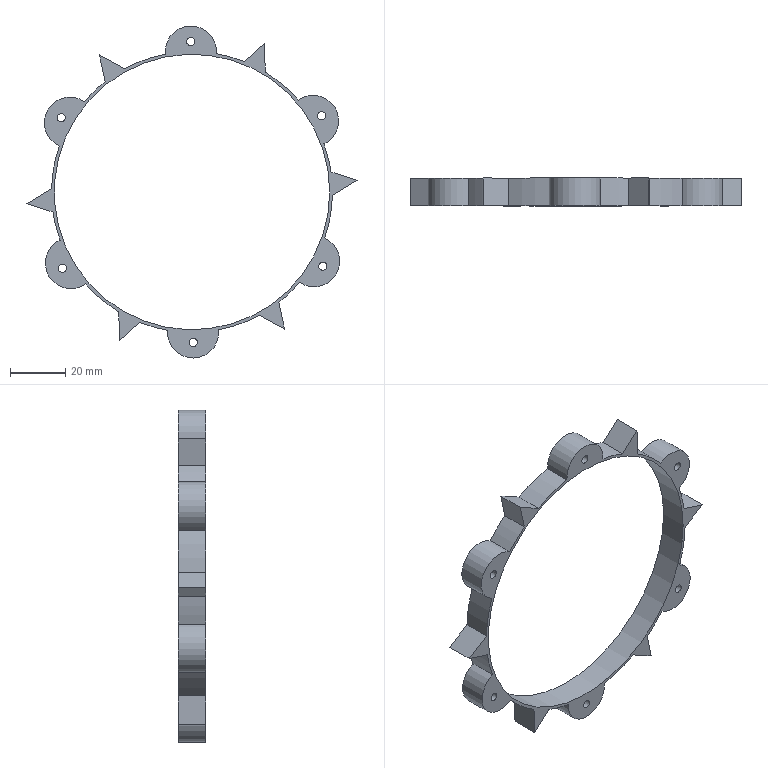Part | NX | features DATUM_CSYS 3, EXTRUDE 2, SKETCH 2 | 1 solid | 39 faces | box 119.85 x 10 x 120.564 mm | volume 13504 mm3 | cylinder 25 | plane 14 | commonest cylinder face diameters 102 x12 3 x6 18.567 x6 100 x1
STEP:
#1=CARTESIAN_POINT('',(-50.984,0.,1.273));
#2=VERTEX_POINT('',#1);
#3=CARTESIAN_POINT('',(-59.925,0.,-4.222));
#4=VERTEX_POINT('',#3);
#5=CARTESIAN_POINT('',(-50.984,0.,1.273));
#6=DIRECTION('',(-0.852,0.,-0.5236));
#7=VECTOR('',#6,1000.);
#8=LINE('',#5,#7);
#9=EDGE_CURVE('',#2,#4,#8,.T.);
#10=ORIENTED_EDGE('',*,*,#9,.T.);
#11=CARTESIAN_POINT('',(-59.925,-10.,-4.222));
#12=VERTEX_POINT('',#11);
#13=CARTESIAN_POINT('',(-59.925,-10.,-4.222));
#14=DIRECTION('',(0.,1.,0.));
#15=VECTOR('',#14,1000.);
#16=LINE('',#13,#15);
#17=EDGE_CURVE('',#12,#4,#16,.T.);
#18=ORIENTED_EDGE('',*,*,#17,.F.);
#19=CARTESIAN_POINT('',(-50.984,-10.,1.273));
#20=VERTEX_POINT('',#19);
#21=CARTESIAN_POINT('',(-50.984,-10.,1.273));
#22=DIRECTION('',(-0.852,0.,-0.5236));
#23=VECTOR('',#22,1000.);
#24=LINE('',#21,#23);
#25=EDGE_CURVE('',#20,#12,#24,.T.);
#26=ORIENTED_EDGE('',*,*,#25,.F.);
#27=CARTESIAN_POINT('',(-50.984,-10.,1.273));
#28=DIRECTION('',(0.,1.,0.));
#29=VECTOR('',#28,1000.);
#30=LINE('',#27,#29);
#31=EDGE_CURVE('',#20,#2,#30,.T.);
#32=ORIENTED_EDGE('',*,*,#31,.T.);
#33=EDGE_LOOP('',(#10,#18,#26,#32));
#34=FACE_BOUND('',#33,.T.);
#35=CARTESIAN_POINT('',(-50.984,-10.,1.273));
#36=DIRECTION('',(0.5236,0.,-0.852));
#37=DIRECTION('',(-0.852,0.,-0.5236));
#38=AXIS2_PLACEMENT_3D('',#35,#36,#37);
#39=PLANE('',#38);
#40=ADVANCED_FACE('',(#34),#39,.F.);
#41=CARTESIAN_POINT('',(-50.476,0.,-7.292));
#42=VERTEX_POINT('',#41);
#43=CARTESIAN_POINT('',(-59.925,0.,-4.222));
#44=DIRECTION('',(0.9511,0.,-0.309));
#45=VECTOR('',#44,1000.);
#46=LINE('',#43,#45);
#47=EDGE_CURVE('',#4,#42,#46,.T.);
#48=ORIENTED_EDGE('',*,*,#47,.T.);
#49=CARTESIAN_POINT('',(-50.476,-10.,-7.292));
#50=VERTEX_POINT('',#49);
#51=CARTESIAN_POINT('',(-50.476,-10.,-7.292));
#52=DIRECTION('',(0.,1.,0.));
#53=VECTOR('',#52,1000.);
#54=LINE('',#51,#53);
#55=EDGE_CURVE('',#50,#42,#54,.T.);
#56=ORIENTED_EDGE('',*,*,#55,.F.);
#57=CARTESIAN_POINT('',(-59.925,-10.,-4.222));
#58=DIRECTION('',(0.9511,0.,-0.309));
#59=VECTOR('',#58,1000.);
#60=LINE('',#57,#59);
#61=EDGE_CURVE('',#12,#50,#60,.T.);
#62=ORIENTED_EDGE('',*,*,#61,.F.);
#63=ORIENTED_EDGE('',*,*,#17,.T.);
#64=EDGE_LOOP('',(#48,#56,#62,#63));
#65=FACE_BOUND('',#64,.T.);
#66=CARTESIAN_POINT('',(-59.925,-10.,-4.222));
#67=DIRECTION('',(0.309,0.,0.9511));
#68=DIRECTION('',(0.9511,0.,-0.309));
#69=AXIS2_PLACEMENT_3D('',#66,#67,#68);
#70=PLANE('',#69);
#71=ADVANCED_FACE('',(#65),#70,.F.);
#72=CARTESIAN_POINT('',(-47.922,0.,-17.449));
#73=VERTEX_POINT('',#72);
#74=CARTESIAN_POINT('',(0.,0.,0.));
#75=DIRECTION('',(0.,-1.,0.));
#76=DIRECTION('',(1.,0.,0.));
#77=AXIS2_PLACEMENT_3D('',#74,#75,#76);
#78=CIRCLE('',#77,51.);
#79=EDGE_CURVE('',#42,#73,#78,.T.);
#80=ORIENTED_EDGE('',*,*,#79,.T.);
#81=CARTESIAN_POINT('',(-47.922,-10.,-17.449));
#82=VERTEX_POINT('',#81);
#83=CARTESIAN_POINT('',(-47.922,-10.,-17.449));
#84=DIRECTION('',(0.,1.,0.));
#85=VECTOR('',#84,1000.);
#86=LINE('',#83,#85);
#87=EDGE_CURVE('',#82,#73,#86,.T.);
#88=ORIENTED_EDGE('',*,*,#87,.F.);
#89=CARTESIAN_POINT('',(0.,-10.,0.));
#90=DIRECTION('',(0.,-1.,0.));
#91=DIRECTION('',(1.,0.,0.));
#92=AXIS2_PLACEMENT_3D('',#89,#90,#91);
#93=CIRCLE('',#92,51.);
#94=EDGE_CURVE('',#50,#82,#93,.T.);
#95=ORIENTED_EDGE('',*,*,#94,.F.);
#96=ORIENTED_EDGE('',*,*,#55,.T.);
#97=EDGE_LOOP('',(#80,#88,#95,#96));
#98=FACE_BOUND('',#97,.T.);
#99=CARTESIAN_POINT('',(0.,-10.,0.));
#100=DIRECTION('',(0.,1.,0.));
#101=DIRECTION('',(0.,0.,1.));
#102=AXIS2_PLACEMENT_3D('',#99,#100,#101);
#103=CYLINDRICAL_SURFACE('',#102,51.);
#104=ADVANCED_FACE('',(#98),#103,.T.);
#105=CARTESIAN_POINT('',(-38.551,0.,-33.388));
#106=VERTEX_POINT('',#105);
#107=CARTESIAN_POINT('',(-43.965,0.,-25.847));
#108=DIRECTION('',(0.,-1.,0.));
#109=DIRECTION('',(-0.5,0.,0.866));
#110=AXIS2_PLACEMENT_3D('',#107,#108,#109);
#111=CIRCLE('',#110,9.283);
#112=EDGE_CURVE('',#73,#106,#111,.T.);
#113=ORIENTED_EDGE('',*,*,#112,.T.);
#114=CARTESIAN_POINT('',(-38.551,-10.,-33.388));
#115=VERTEX_POINT('',#114);
#116=CARTESIAN_POINT('',(-38.551,-10.,-33.388));
#117=DIRECTION('',(0.,1.,0.));
#118=VECTOR('',#117,1000.);
#119=LINE('',#116,#118);
#120=EDGE_CURVE('',#115,#106,#119,.T.);
#121=ORIENTED_EDGE('',*,*,#120,.F.);
#122=CARTESIAN_POINT('',(-43.965,-10.,-25.847));
#123=DIRECTION('',(0.,-1.,0.));
#124=DIRECTION('',(-0.5,0.,0.866));
#125=AXIS2_PLACEMENT_3D('',#122,#123,#124);
#126=CIRCLE('',#125,9.283);
#127=EDGE_CURVE('',#82,#115,#126,.T.);
#128=ORIENTED_EDGE('',*,*,#127,.F.);
#129=ORIENTED_EDGE('',*,*,#87,.T.);
#130=EDGE_LOOP('',(#113,#121,#128,#129));
#131=FACE_BOUND('',#130,.T.);
#132=CARTESIAN_POINT('',(-43.965,-10.,-25.847));
#133=DIRECTION('',(0.,1.,0.));
#134=DIRECTION('',(0.,0.,1.));
#135=AXIS2_PLACEMENT_3D('',#132,#133,#134);
#136=CYLINDRICAL_SURFACE('',#135,9.283);
#137=ADVANCED_FACE('',(#131),#136,.T.);
#138=CARTESIAN_POINT('',(-26.594,0.,-43.517));
#139=VERTEX_POINT('',#138);
#140=CARTESIAN_POINT('',(0.,0.,0.));
#141=DIRECTION('',(0.,-1.,0.));
#142=DIRECTION('',(1.,0.,0.));
#143=AXIS2_PLACEMENT_3D('',#140,#141,#142);
#144=CIRCLE('',#143,51.);
#145=EDGE_CURVE('',#106,#139,#144,.T.);
#146=ORIENTED_EDGE('',*,*,#145,.T.);
#147=CARTESIAN_POINT('',(-26.594,-10.,-43.517));
#148=VERTEX_POINT('',#147);
#149=CARTESIAN_POINT('',(-26.594,-10.,-43.517));
#150=DIRECTION('',(0.,1.,0.));
#151=VECTOR('',#150,1000.);
#152=LINE('',#149,#151);
#153=EDGE_CURVE('',#148,#139,#152,.T.);
#154=ORIENTED_EDGE('',*,*,#153,.F.);
#155=CARTESIAN_POINT('',(0.,-10.,0.));
#156=DIRECTION('',(0.,-1.,0.));
#157=DIRECTION('',(1.,0.,0.));
#158=AXIS2_PLACEMENT_3D('',#155,#156,#157);
#159=CIRCLE('',#158,51.);
#160=EDGE_CURVE('',#115,#148,#159,.T.);
#161=ORIENTED_EDGE('',*,*,#160,.F.);
#162=ORIENTED_EDGE('',*,*,#120,.T.);
#163=EDGE_LOOP('',(#146,#154,#161,#162));
#164=FACE_BOUND('',#163,.T.);
#165=CARTESIAN_POINT('',(0.,-10.,0.));
#166=DIRECTION('',(0.,1.,0.));
#167=DIRECTION('',(0.,0.,1.));
#168=AXIS2_PLACEMENT_3D('',#165,#166,#167);
#169=CYLINDRICAL_SURFACE('',#168,51.);
#170=ADVANCED_FACE('',(#164),#169,.T.);
#171=CARTESIAN_POINT('',(-26.306,0.,-54.007));
#172=VERTEX_POINT('',#171);
#173=CARTESIAN_POINT('',(-26.594,0.,-43.517));
#174=DIRECTION('',(0.02744,0.,-0.9996));
#175=VECTOR('',#174,1000.);
#176=LINE('',#173,#175);
#177=EDGE_CURVE('',#139,#172,#176,.T.);
#178=ORIENTED_EDGE('',*,*,#177,.T.);
#179=CARTESIAN_POINT('',(-26.306,-10.,-54.007));
#180=VERTEX_POINT('',#179);
#181=CARTESIAN_POINT('',(-26.306,-10.,-54.007));
#182=DIRECTION('',(0.,1.,0.));
#183=VECTOR('',#182,1000.);
#184=LINE('',#181,#183);
#185=EDGE_CURVE('',#180,#172,#184,.T.);
#186=ORIENTED_EDGE('',*,*,#185,.F.);
#187=CARTESIAN_POINT('',(-26.594,-10.,-43.517));
#188=DIRECTION('',(0.02744,0.,-0.9996));
#189=VECTOR('',#188,1000.);
#190=LINE('',#187,#189);
#191=EDGE_CURVE('',#148,#180,#190,.T.);
#192=ORIENTED_EDGE('',*,*,#191,.F.);
#193=ORIENTED_EDGE('',*,*,#153,.T.);
#194=EDGE_LOOP('',(#178,#186,#192,#193));
#195=FACE_BOUND('',#194,.T.);
#196=CARTESIAN_POINT('',(-26.594,-10.,-43.517));
#197=DIRECTION('',(0.9996,0.,0.02744));
#198=DIRECTION('',(0.02744,0.,-0.9996));
#199=AXIS2_PLACEMENT_3D('',#196,#197,#198);
#200=PLANE('',#199);
#201=ADVANCED_FACE('',(#195),#200,.F.);
#202=CARTESIAN_POINT('',(-18.923,0.,-47.359));
#203=VERTEX_POINT('',#202);
#204=CARTESIAN_POINT('',(-26.306,0.,-54.007));
#205=DIRECTION('',(0.7431,0.,0.6691));
#206=VECTOR('',#205,1000.);
#207=LINE('',#204,#206);
#208=EDGE_CURVE('',#172,#203,#207,.T.);
#209=ORIENTED_EDGE('',*,*,#208,.T.);
#210=CARTESIAN_POINT('',(-18.923,-10.,-47.359));
#211=VERTEX_POINT('',#210);
#212=CARTESIAN_POINT('',(-18.923,-10.,-47.359));
#213=DIRECTION('',(0.,1.,0.));
#214=VECTOR('',#213,1000.);
#215=LINE('',#212,#214);
#216=EDGE_CURVE('',#211,#203,#215,.T.);
#217=ORIENTED_EDGE('',*,*,#216,.F.);
#218=CARTESIAN_POINT('',(-26.306,-10.,-54.007));
#219=DIRECTION('',(0.7431,0.,0.6691));
#220=VECTOR('',#219,1000.);
#221=LINE('',#218,#220);
#222=EDGE_CURVE('',#180,#211,#221,.T.);
#223=ORIENTED_EDGE('',*,*,#222,.F.);
#224=ORIENTED_EDGE('',*,*,#185,.T.);
#225=EDGE_LOOP('',(#209,#217,#223,#224));
#226=FACE_BOUND('',#225,.T.);
#227=CARTESIAN_POINT('',(-26.306,-10.,-54.007));
#228=DIRECTION('',(-0.6691,0.,0.7431));
#229=DIRECTION('',(0.7431,0.,0.6691));
#230=AXIS2_PLACEMENT_3D('',#227,#228,#229);
#231=PLANE('',#230);
#232=ADVANCED_FACE('',(#226),#231,.F.);
#233=CARTESIAN_POINT('',(-8.85,0.,-50.226));
#234=VERTEX_POINT('',#233);
#235=CARTESIAN_POINT('',(0.,0.,0.));
#236=DIRECTION('',(0.,-1.,0.));
#237=DIRECTION('',(1.,0.,0.));
#238=AXIS2_PLACEMENT_3D('',#235,#236,#237);
#239=CIRCLE('',#238,51.);
#240=EDGE_CURVE('',#203,#234,#239,.T.);
#241=ORIENTED_EDGE('',*,*,#240,.T.);
#242=CARTESIAN_POINT('',(-8.85,-10.,-50.226));
#243=VERTEX_POINT('',#242);
#244=CARTESIAN_POINT('',(-8.85,-10.,-50.226));
#245=DIRECTION('',(0.,1.,0.));
#246=VECTOR('',#245,1000.);
#247=LINE('',#244,#246);
#248=EDGE_CURVE('',#243,#234,#247,.T.);
#249=ORIENTED_EDGE('',*,*,#248,.F.);
#250=CARTESIAN_POINT('',(0.,-10.,0.));
#251=DIRECTION('',(0.,-1.,0.));
#252=DIRECTION('',(1.,0.,0.));
#253=AXIS2_PLACEMENT_3D('',#250,#251,#252);
#254=CIRCLE('',#253,51.);
#255=EDGE_CURVE('',#211,#243,#254,.T.);
#256=ORIENTED_EDGE('',*,*,#255,.F.);
#257=ORIENTED_EDGE('',*,*,#216,.T.);
#258=EDGE_LOOP('',(#241,#249,#256,#257));
#259=FACE_BOUND('',#258,.T.);
#260=CARTESIAN_POINT('',(0.,-10.,0.));
#261=DIRECTION('',(0.,1.,0.));
#262=DIRECTION('',(0.,0.,1.));
#263=AXIS2_PLACEMENT_3D('',#260,#261,#262);
#264=CYLINDRICAL_SURFACE('',#263,51.);
#265=ADVANCED_FACE('',(#259),#264,.T.);
#266=CARTESIAN_POINT('',(9.64,0.,-50.081));
#267=VERTEX_POINT('',#266);
#268=CARTESIAN_POINT('',(0.4017,0.,-50.998));
#269=DIRECTION('',(0.,-1.,0.));
#270=DIRECTION('',(-1.,0.,0.));
#271=AXIS2_PLACEMENT_3D('',#268,#269,#270);
#272=CIRCLE('',#271,9.283);
#273=EDGE_CURVE('',#234,#267,#272,.T.);
#274=ORIENTED_EDGE('',*,*,#273,.T.);
#275=CARTESIAN_POINT('',(9.64,-10.,-50.081));
#276=VERTEX_POINT('',#275);
#277=CARTESIAN_POINT('',(9.64,-10.,-50.081));
#278=DIRECTION('',(0.,1.,0.));
#279=VECTOR('',#278,1000.);
#280=LINE('',#277,#279);
#281=EDGE_CURVE('',#276,#267,#280,.T.);
#282=ORIENTED_EDGE('',*,*,#281,.F.);
#283=CARTESIAN_POINT('',(0.4017,-10.,-50.998));
#284=DIRECTION('',(0.,-1.,0.));
#285=DIRECTION('',(-1.,0.,0.));
#286=AXIS2_PLACEMENT_3D('',#283,#284,#285);
#287=CIRCLE('',#286,9.283);
#288=EDGE_CURVE('',#243,#276,#287,.T.);
#289=ORIENTED_EDGE('',*,*,#288,.F.);
#290=ORIENTED_EDGE('',*,*,#248,.T.);
#291=EDGE_LOOP('',(#274,#282,#289,#290));
#292=FACE_BOUND('',#291,.T.);
#293=CARTESIAN_POINT('',(0.4017,-10.,-50.998));
#294=DIRECTION('',(0.,1.,0.));
#295=DIRECTION('',(0.,0.,1.));
#296=AXIS2_PLACEMENT_3D('',#293,#294,#295);
#297=CYLINDRICAL_SURFACE('',#296,9.283);
#298=ADVANCED_FACE('',(#292),#297,.T.);
#299=CARTESIAN_POINT('',(24.39,0.,-44.79));
#300=VERTEX_POINT('',#299);
#301=CARTESIAN_POINT('',(0.,0.,0.));
#302=DIRECTION('',(0.,-1.,0.));
#303=DIRECTION('',(1.,0.,0.));
#304=AXIS2_PLACEMENT_3D('',#301,#302,#303);
#305=CIRCLE('',#304,51.);
#306=EDGE_CURVE('',#267,#300,#305,.T.);
#307=ORIENTED_EDGE('',*,*,#306,.T.);
#308=CARTESIAN_POINT('',(24.39,-10.,-44.79));
#309=VERTEX_POINT('',#308);
#310=CARTESIAN_POINT('',(24.39,-10.,-44.79));
#311=DIRECTION('',(0.,1.,0.));
#312=VECTOR('',#311,1000.);
#313=LINE('',#310,#312);
#314=EDGE_CURVE('',#309,#300,#313,.T.);
#315=ORIENTED_EDGE('',*,*,#314,.F.);
#316=CARTESIAN_POINT('',(0.,-10.,0.));
#317=DIRECTION('',(0.,-1.,0.));
#318=DIRECTION('',(1.,0.,0.));
#319=AXIS2_PLACEMENT_3D('',#316,#317,#318);
#320=CIRCLE('',#319,51.);
#321=EDGE_CURVE('',#276,#309,#320,.T.);
#322=ORIENTED_EDGE('',*,*,#321,.F.);
#323=ORIENTED_EDGE('',*,*,#281,.T.);
#324=EDGE_LOOP('',(#307,#315,#322,#323));
#325=FACE_BOUND('',#324,.T.);
#326=CARTESIAN_POINT('',(0.,-10.,0.));
#327=DIRECTION('',(0.,1.,0.));
#328=DIRECTION('',(0.,0.,1.));
#329=AXIS2_PLACEMENT_3D('',#326,#327,#328);
#330=CYLINDRICAL_SURFACE('',#329,51.);
#331=ADVANCED_FACE('',(#325),#330,.T.);
#332=CARTESIAN_POINT('',(33.619,0.,-49.786));
#333=VERTEX_POINT('',#332);
#334=CARTESIAN_POINT('',(24.39,0.,-44.79));
#335=DIRECTION('',(0.8794,0.,-0.476));
#336=VECTOR('',#335,1000.);
#337=LINE('',#334,#336);
#338=EDGE_CURVE('',#300,#333,#337,.T.);
#339=ORIENTED_EDGE('',*,*,#338,.T.);
#340=CARTESIAN_POINT('',(33.619,-10.,-49.786));
#341=VERTEX_POINT('',#340);
#342=CARTESIAN_POINT('',(33.619,-10.,-49.786));
#343=DIRECTION('',(0.,1.,0.));
#344=VECTOR('',#343,1000.);
#345=LINE('',#342,#344);
#346=EDGE_CURVE('',#341,#333,#345,.T.);
#347=ORIENTED_EDGE('',*,*,#346,.F.);
#348=CARTESIAN_POINT('',(24.39,-10.,-44.79));
#349=DIRECTION('',(0.8794,0.,-0.476));
#350=VECTOR('',#349,1000.);
#351=LINE('',#348,#350);
#352=EDGE_CURVE('',#309,#341,#351,.T.);
#353=ORIENTED_EDGE('',*,*,#352,.F.);
#354=ORIENTED_EDGE('',*,*,#314,.T.);
#355=EDGE_LOOP('',(#339,#347,#353,#354));
#356=FACE_BOUND('',#355,.T.);
#357=CARTESIAN_POINT('',(24.39,-10.,-44.79));
#358=DIRECTION('',(0.476,0.,0.8794));
#359=DIRECTION('',(0.8794,0.,-0.476));
#360=AXIS2_PLACEMENT_3D('',#357,#358,#359);
#361=PLANE('',#360);
#362=ADVANCED_FACE('',(#356),#361,.F.);
#363=CARTESIAN_POINT('',(31.553,0.,-40.068));
#364=VERTEX_POINT('',#363);
#365=CARTESIAN_POINT('',(33.619,0.,-49.786));
#366=DIRECTION('',(-0.2079,0.,0.9781));
#367=VECTOR('',#366,1000.);
#368=LINE('',#365,#367);
#369=EDGE_CURVE('',#333,#364,#368,.T.);
#370=ORIENTED_EDGE('',*,*,#369,.T.);
#371=CARTESIAN_POINT('',(31.553,-10.,-40.068));
#372=VERTEX_POINT('',#371);
#373=CARTESIAN_POINT('',(31.553,-10.,-40.068));
#374=DIRECTION('',(0.,1.,0.));
#375=VECTOR('',#374,1000.);
#376=LINE('',#373,#375);
#377=EDGE_CURVE('',#372,#364,#376,.T.);
#378=ORIENTED_EDGE('',*,*,#377,.F.);
#379=CARTESIAN_POINT('',(33.619,-10.,-49.786));
#380=DIRECTION('',(-0.2079,0.,0.9781));
#381=VECTOR('',#380,1000.);
#382=LINE('',#379,#381);
#383=EDGE_CURVE('',#341,#372,#382,.T.);
#384=ORIENTED_EDGE('',*,*,#383,.F.);
#385=ORIENTED_EDGE('',*,*,#346,.T.);
#386=EDGE_LOOP('',(#370,#378,#384,#385));
#387=FACE_BOUND('',#386,.T.);
#388=CARTESIAN_POINT('',(33.619,-10.,-49.786));
#389=DIRECTION('',(-0.9781,0.,-0.2079));
#390=DIRECTION('',(-0.2079,0.,0.9781));
#391=AXIS2_PLACEMENT_3D('',#388,#389,#390);
#392=PLANE('',#391);
#393=ADVANCED_FACE('',(#387),#392,.F.);
#394=CARTESIAN_POINT('',(39.073,0.,-32.777));
#395=VERTEX_POINT('',#394);
#396=CARTESIAN_POINT('',(0.,0.,0.));
#397=DIRECTION('',(0.,-1.,0.));
#398=DIRECTION('',(1.,0.,0.));
#399=AXIS2_PLACEMENT_3D('',#396,#397,#398);
#400=CIRCLE('',#399,51.);
#401=EDGE_CURVE('',#364,#395,#400,.T.);
#402=ORIENTED_EDGE('',*,*,#401,.T.);
#403=CARTESIAN_POINT('',(39.073,-10.,-32.777));
#404=VERTEX_POINT('',#403);
#405=CARTESIAN_POINT('',(39.073,-10.,-32.777));
#406=DIRECTION('',(0.,1.,0.));
#407=VECTOR('',#406,1000.);
#408=LINE('',#405,#407);
#409=EDGE_CURVE('',#404,#395,#408,.T.);
#410=ORIENTED_EDGE('',*,*,#409,.F.);
#411=CARTESIAN_POINT('',(0.,-10.,0.));
#412=DIRECTION('',(0.,-1.,0.));
#413=DIRECTION('',(1.,0.,0.));
#414=AXIS2_PLACEMENT_3D('',#411,#412,#413);
#415=CIRCLE('',#414,51.);
#416=EDGE_CURVE('',#372,#404,#415,.T.);
#417=ORIENTED_EDGE('',*,*,#416,.F.);
#418=ORIENTED_EDGE('',*,*,#377,.T.);
#419=EDGE_LOOP('',(#402,#410,#417,#418));
#420=FACE_BOUND('',#419,.T.);
#421=CARTESIAN_POINT('',(0.,-10.,0.));
#422=DIRECTION('',(0.,1.,0.));
#423=DIRECTION('',(0.,0.,1.));
#424=AXIS2_PLACEMENT_3D('',#421,#422,#423);
#425=CYLINDRICAL_SURFACE('',#424,51.);
#426=ADVANCED_FACE('',(#420),#425,.T.);
#427=CARTESIAN_POINT('',(48.191,0.,-16.692));
#428=VERTEX_POINT('',#427);
#429=CARTESIAN_POINT('',(44.367,0.,-25.151));
#430=DIRECTION('',(0.,-1.,0.));
#431=DIRECTION('',(-0.5,0.,-0.866));
#432=AXIS2_PLACEMENT_3D('',#429,#430,#431);
#433=CIRCLE('',#432,9.283);
#434=EDGE_CURVE('',#395,#428,#433,.T.);
#435=ORIENTED_EDGE('',*,*,#434,.T.);
#436=CARTESIAN_POINT('',(48.191,-10.,-16.692));
#437=VERTEX_POINT('',#436);
#438=CARTESIAN_POINT('',(48.191,-10.,-16.692));
#439=DIRECTION('',(0.,1.,0.));
#440=VECTOR('',#439,1000.);
#441=LINE('',#438,#440);
#442=EDGE_CURVE('',#437,#428,#441,.T.);
#443=ORIENTED_EDGE('',*,*,#442,.F.);
#444=CARTESIAN_POINT('',(44.367,-10.,-25.151));
#445=DIRECTION('',(0.,-1.,0.));
#446=DIRECTION('',(-0.5,0.,-0.866));
#447=AXIS2_PLACEMENT_3D('',#444,#445,#446);
#448=CIRCLE('',#447,9.283);
#449=EDGE_CURVE('',#404,#437,#448,.T.);
#450=ORIENTED_EDGE('',*,*,#449,.F.);
#451=ORIENTED_EDGE('',*,*,#409,.T.);
#452=EDGE_LOOP('',(#435,#443,#450,#451));
#453=FACE_BOUND('',#452,.T.);
#454=CARTESIAN_POINT('',(44.367,-10.,-25.151));
#455=DIRECTION('',(0.,1.,0.));
#456=DIRECTION('',(0.,0.,1.));
#457=AXIS2_PLACEMENT_3D('',#454,#455,#456);
#458=CYLINDRICAL_SURFACE('',#457,9.283);
#459=ADVANCED_FACE('',(#453),#458,.T.);
#460=CARTESIAN_POINT('',(50.984,0.,-1.273));
#461=VERTEX_POINT('',#460);
#462=CARTESIAN_POINT('',(0.,0.,0.));
#463=DIRECTION('',(0.,-1.,0.));
#464=DIRECTION('',(1.,0.,0.));
#465=AXIS2_PLACEMENT_3D('',#462,#463,#464);
#466=CIRCLE('',#465,51.);
#467=EDGE_CURVE('',#428,#461,#466,.T.);
#468=ORIENTED_EDGE('',*,*,#467,.T.);
#469=CARTESIAN_POINT('',(50.984,-10.,-1.273));
#470=VERTEX_POINT('',#469);
#471=CARTESIAN_POINT('',(50.984,-10.,-1.273));
#472=DIRECTION('',(0.,1.,0.));
#473=VECTOR('',#472,1000.);
#474=LINE('',#471,#473);
#475=EDGE_CURVE('',#470,#461,#474,.T.);
#476=ORIENTED_EDGE('',*,*,#475,.F.);
#477=CARTESIAN_POINT('',(0.,-10.,0.));
#478=DIRECTION('',(0.,-1.,0.));
#479=DIRECTION('',(1.,0.,0.));
#480=AXIS2_PLACEMENT_3D('',#477,#478,#479);
#481=CIRCLE('',#480,51.);
#482=EDGE_CURVE('',#437,#470,#481,.T.);
#483=ORIENTED_EDGE('',*,*,#482,.F.);
#484=ORIENTED_EDGE('',*,*,#442,.T.);
#485=EDGE_LOOP('',(#468,#476,#483,#484));
#486=FACE_BOUND('',#485,.T.);
#487=CARTESIAN_POINT('',(0.,-10.,0.));
#488=DIRECTION('',(0.,1.,0.));
#489=DIRECTION('',(0.,0.,1.));
#490=AXIS2_PLACEMENT_3D('',#487,#488,#489);
#491=CYLINDRICAL_SURFACE('',#490,51.);
#492=ADVANCED_FACE('',(#486),#491,.T.);
#493=CARTESIAN_POINT('',(59.925,0.,4.222));
#494=VERTEX_POINT('',#493);
#495=CARTESIAN_POINT('',(50.984,0.,-1.273));
#496=DIRECTION('',(0.852,0.,0.5236));
#497=VECTOR('',#496,1000.);
#498=LINE('',#495,#497);
#499=EDGE_CURVE('',#461,#494,#498,.T.);
#500=ORIENTED_EDGE('',*,*,#499,.T.);
#501=CARTESIAN_POINT('',(59.925,-10.,4.222));
#502=VERTEX_POINT('',#501);
#503=CARTESIAN_POINT('',(59.925,-10.,4.222));
#504=DIRECTION('',(0.,1.,0.));
#505=VECTOR('',#504,1000.);
#506=LINE('',#503,#505);
#507=EDGE_CURVE('',#502,#494,#506,.T.);
#508=ORIENTED_EDGE('',*,*,#507,.F.);
#509=CARTESIAN_POINT('',(50.984,-10.,-1.273));
#510=DIRECTION('',(0.852,0.,0.5236));
#511=VECTOR('',#510,1000.);
#512=LINE('',#509,#511);
#513=EDGE_CURVE('',#470,#502,#512,.T.);
#514=ORIENTED_EDGE('',*,*,#513,.F.);
#515=ORIENTED_EDGE('',*,*,#475,.T.);
#516=EDGE_LOOP('',(#500,#508,#514,#515));
#517=FACE_BOUND('',#516,.T.);
#518=CARTESIAN_POINT('',(50.984,-10.,-1.273));
#519=DIRECTION('',(-0.5236,0.,0.852));
#520=DIRECTION('',(0.852,0.,0.5236));
#521=AXIS2_PLACEMENT_3D('',#518,#519,#520);
#522=PLANE('',#521);
#523=ADVANCED_FACE('',(#517),#522,.F.);
#524=CARTESIAN_POINT('',(50.476,0.,7.292));
#525=VERTEX_POINT('',#524);
#526=CARTESIAN_POINT('',(59.925,0.,4.222));
#527=DIRECTION('',(-0.9511,0.,0.309));
#528=VECTOR('',#527,1000.);
#529=LINE('',#526,#528);
#530=EDGE_CURVE('',#494,#525,#529,.T.);
#531=ORIENTED_EDGE('',*,*,#530,.T.);
#532=CARTESIAN_POINT('',(50.476,-10.,7.292));
#533=VERTEX_POINT('',#532);
#534=CARTESIAN_POINT('',(50.476,-10.,7.292));
#535=DIRECTION('',(0.,1.,0.));
#536=VECTOR('',#535,1000.);
#537=LINE('',#534,#536);
#538=EDGE_CURVE('',#533,#525,#537,.T.);
#539=ORIENTED_EDGE('',*,*,#538,.F.);
#540=CARTESIAN_POINT('',(59.925,-10.,4.222));
#541=DIRECTION('',(-0.9511,0.,0.309));
#542=VECTOR('',#541,1000.);
#543=LINE('',#540,#542);
#544=EDGE_CURVE('',#502,#533,#543,.T.);
#545=ORIENTED_EDGE('',*,*,#544,.F.);
#546=ORIENTED_EDGE('',*,*,#507,.T.);
#547=EDGE_LOOP('',(#531,#539,#545,#546));
#548=FACE_BOUND('',#547,.T.);
#549=CARTESIAN_POINT('',(59.925,-10.,4.222));
#550=DIRECTION('',(-0.309,0.,-0.9511));
#551=DIRECTION('',(-0.9511,0.,0.309));
#552=AXIS2_PLACEMENT_3D('',#549,#550,#551);
#553=PLANE('',#552);
#554=ADVANCED_FACE('',(#548),#553,.F.);
#555=CARTESIAN_POINT('',(47.922,0.,17.449));
#556=VERTEX_POINT('',#555);
#557=CARTESIAN_POINT('',(0.,0.,0.));
#558=DIRECTION('',(0.,-1.,0.));
#559=DIRECTION('',(1.,0.,0.));
#560=AXIS2_PLACEMENT_3D('',#557,#558,#559);
#561=CIRCLE('',#560,51.);
#562=EDGE_CURVE('',#525,#556,#561,.T.);
#563=ORIENTED_EDGE('',*,*,#562,.T.);
#564=CARTESIAN_POINT('',(47.922,-10.,17.449));
#565=VERTEX_POINT('',#564);
#566=CARTESIAN_POINT('',(47.922,-10.,17.449));
#567=DIRECTION('',(0.,1.,0.));
#568=VECTOR('',#567,1000.);
#569=LINE('',#566,#568);
#570=EDGE_CURVE('',#565,#556,#569,.T.);
#571=ORIENTED_EDGE('',*,*,#570,.F.);
#572=CARTESIAN_POINT('',(0.,-10.,0.));
#573=DIRECTION('',(0.,-1.,0.));
#574=DIRECTION('',(1.,0.,0.));
#575=AXIS2_PLACEMENT_3D('',#572,#573,#574);
#576=CIRCLE('',#575,51.);
#577=EDGE_CURVE('',#533,#565,#576,.T.);
#578=ORIENTED_EDGE('',*,*,#577,.F.);
#579=ORIENTED_EDGE('',*,*,#538,.T.);
#580=EDGE_LOOP('',(#563,#571,#578,#579));
#581=FACE_BOUND('',#580,.T.);
#582=CARTESIAN_POINT('',(0.,-10.,0.));
#583=DIRECTION('',(0.,1.,0.));
#584=DIRECTION('',(0.,0.,1.));
#585=AXIS2_PLACEMENT_3D('',#582,#583,#584);
#586=CYLINDRICAL_SURFACE('',#585,51.);
#587=ADVANCED_FACE('',(#581),#586,.T.);
#588=CARTESIAN_POINT('',(38.551,0.,33.388));
#589=VERTEX_POINT('',#588);
#590=CARTESIAN_POINT('',(43.965,0.,25.847));
#591=DIRECTION('',(0.,-1.,0.));
#592=DIRECTION('',(0.5,0.,-0.866));
#593=AXIS2_PLACEMENT_3D('',#590,#591,#592);
#594=CIRCLE('',#593,9.283);
#595=EDGE_CURVE('',#556,#589,#594,.T.);
#596=ORIENTED_EDGE('',*,*,#595,.T.);
#597=CARTESIAN_POINT('',(38.551,-10.,33.388));
#598=VERTEX_POINT('',#597);
#599=CARTESIAN_POINT('',(38.551,-10.,33.388));
#600=DIRECTION('',(0.,1.,0.));
#601=VECTOR('',#600,1000.);
#602=LINE('',#599,#601);
#603=EDGE_CURVE('',#598,#589,#602,.T.);
#604=ORIENTED_EDGE('',*,*,#603,.F.);
#605=CARTESIAN_POINT('',(43.965,-10.,25.847));
#606=DIRECTION('',(0.,-1.,0.));
#607=DIRECTION('',(0.5,0.,-0.866));
#608=AXIS2_PLACEMENT_3D('',#605,#606,#607);
#609=CIRCLE('',#608,9.283);
#610=EDGE_CURVE('',#565,#598,#609,.T.);
#611=ORIENTED_EDGE('',*,*,#610,.F.);
#612=ORIENTED_EDGE('',*,*,#570,.T.);
#613=EDGE_LOOP('',(#596,#604,#611,#612));
#614=FACE_BOUND('',#613,.T.);
#615=CARTESIAN_POINT('',(43.965,-10.,25.847));
#616=DIRECTION('',(0.,1.,0.));
#617=DIRECTION('',(0.,0.,1.));
#618=AXIS2_PLACEMENT_3D('',#615,#616,#617);
#619=CYLINDRICAL_SURFACE('',#618,9.283);
#620=ADVANCED_FACE('',(#614),#619,.T.);
#621=CARTESIAN_POINT('',(26.594,0.,43.517));
#622=VERTEX_POINT('',#621);
#623=CARTESIAN_POINT('',(0.,0.,0.));
#624=DIRECTION('',(0.,-1.,0.));
#625=DIRECTION('',(1.,0.,0.));
#626=AXIS2_PLACEMENT_3D('',#623,#624,#625);
#627=CIRCLE('',#626,51.);
#628=EDGE_CURVE('',#589,#622,#627,.T.);
#629=ORIENTED_EDGE('',*,*,#628,.T.);
#630=CARTESIAN_POINT('',(26.594,-10.,43.517));
#631=VERTEX_POINT('',#630);
#632=CARTESIAN_POINT('',(26.594,-10.,43.517));
#633=DIRECTION('',(0.,1.,0.));
#634=VECTOR('',#633,1000.);
#635=LINE('',#632,#634);
#636=EDGE_CURVE('',#631,#622,#635,.T.);
#637=ORIENTED_EDGE('',*,*,#636,.F.);
#638=CARTESIAN_POINT('',(0.,-10.,0.));
#639=DIRECTION('',(0.,-1.,0.));
#640=DIRECTION('',(1.,0.,0.));
#641=AXIS2_PLACEMENT_3D('',#638,#639,#640);
#642=CIRCLE('',#641,51.);
#643=EDGE_CURVE('',#598,#631,#642,.T.);
#644=ORIENTED_EDGE('',*,*,#643,.F.);
#645=ORIENTED_EDGE('',*,*,#603,.T.);
#646=EDGE_LOOP('',(#629,#637,#644,#645));
#647=FACE_BOUND('',#646,.T.);
#648=CARTESIAN_POINT('',(0.,-10.,0.));
#649=DIRECTION('',(0.,1.,0.));
#650=DIRECTION('',(0.,0.,1.));
#651=AXIS2_PLACEMENT_3D('',#648,#649,#650);
#652=CYLINDRICAL_SURFACE('',#651,51.);
#653=ADVANCED_FACE('',(#647),#652,.T.);
#654=CARTESIAN_POINT('',(26.306,0.,54.007));
#655=VERTEX_POINT('',#654);
#656=CARTESIAN_POINT('',(26.594,0.,43.517));
#657=DIRECTION('',(-0.02744,0.,0.9996));
#658=VECTOR('',#657,1000.);
#659=LINE('',#656,#658);
#660=EDGE_CURVE('',#622,#655,#659,.T.);
#661=ORIENTED_EDGE('',*,*,#660,.T.);
#662=CARTESIAN_POINT('',(26.306,-10.,54.007));
#663=VERTEX_POINT('',#662);
#664=CARTESIAN_POINT('',(26.306,-10.,54.007));
#665=DIRECTION('',(0.,1.,0.));
#666=VECTOR('',#665,1000.);
#667=LINE('',#664,#666);
#668=EDGE_CURVE('',#663,#655,#667,.T.);
#669=ORIENTED_EDGE('',*,*,#668,.F.);
#670=CARTESIAN_POINT('',(26.594,-10.,43.517));
#671=DIRECTION('',(-0.02744,0.,0.9996));
#672=VECTOR('',#671,1000.);
#673=LINE('',#670,#672);
#674=EDGE_CURVE('',#631,#663,#673,.T.);
#675=ORIENTED_EDGE('',*,*,#674,.F.);
#676=ORIENTED_EDGE('',*,*,#636,.T.);
#677=EDGE_LOOP('',(#661,#669,#675,#676));
#678=FACE_BOUND('',#677,.T.);
#679=CARTESIAN_POINT('',(26.594,-10.,43.517));
#680=DIRECTION('',(-0.9996,0.,-0.02744));
#681=DIRECTION('',(-0.02744,0.,0.9996));
#682=AXIS2_PLACEMENT_3D('',#679,#680,#681);
#683=PLANE('',#682);
#684=ADVANCED_FACE('',(#678),#683,.F.);
#685=CARTESIAN_POINT('',(18.923,0.,47.359));
#686=VERTEX_POINT('',#685);
#687=CARTESIAN_POINT('',(26.306,0.,54.007));
#688=DIRECTION('',(-0.7431,0.,-0.6691));
#689=VECTOR('',#688,1000.);
#690=LINE('',#687,#689);
#691=EDGE_CURVE('',#655,#686,#690,.T.);
#692=ORIENTED_EDGE('',*,*,#691,.T.);
#693=CARTESIAN_POINT('',(18.923,-10.,47.359));
#694=VERTEX_POINT('',#693);
#695=CARTESIAN_POINT('',(18.923,-10.,47.359));
#696=DIRECTION('',(0.,1.,0.));
#697=VECTOR('',#696,1000.);
#698=LINE('',#695,#697);
#699=EDGE_CURVE('',#694,#686,#698,.T.);
#700=ORIENTED_EDGE('',*,*,#699,.F.);
#701=CARTESIAN_POINT('',(26.306,-10.,54.007));
#702=DIRECTION('',(-0.7431,0.,-0.6691));
#703=VECTOR('',#702,1000.);
#704=LINE('',#701,#703);
#705=EDGE_CURVE('',#663,#694,#704,.T.);
#706=ORIENTED_EDGE('',*,*,#705,.F.);
#707=ORIENTED_EDGE('',*,*,#668,.T.);
#708=EDGE_LOOP('',(#692,#700,#706,#707));
#709=FACE_BOUND('',#708,.T.);
#710=CARTESIAN_POINT('',(26.306,-10.,54.007));
#711=DIRECTION('',(0.6691,0.,-0.7431));
#712=DIRECTION('',(-0.7431,0.,-0.6691));
#713=AXIS2_PLACEMENT_3D('',#710,#711,#712);
#714=PLANE('',#713);
#715=ADVANCED_FACE('',(#709),#714,.F.);
#716=CARTESIAN_POINT('',(8.85,0.,50.226));
#717=VERTEX_POINT('',#716);
#718=CARTESIAN_POINT('',(0.,0.,0.));
#719=DIRECTION('',(0.,-1.,0.));
#720=DIRECTION('',(1.,0.,0.));
#721=AXIS2_PLACEMENT_3D('',#718,#719,#720);
#722=CIRCLE('',#721,51.);
#723=EDGE_CURVE('',#686,#717,#722,.T.);
#724=ORIENTED_EDGE('',*,*,#723,.T.);
#725=CARTESIAN_POINT('',(8.85,-10.,50.226));
#726=VERTEX_POINT('',#725);
#727=CARTESIAN_POINT('',(8.85,-10.,50.226));
#728=DIRECTION('',(0.,1.,0.));
#729=VECTOR('',#728,1000.);
#730=LINE('',#727,#729);
#731=EDGE_CURVE('',#726,#717,#730,.T.);
#732=ORIENTED_EDGE('',*,*,#731,.F.);
#733=CARTESIAN_POINT('',(0.,-10.,0.));
#734=DIRECTION('',(0.,-1.,0.));
#735=DIRECTION('',(1.,0.,0.));
#736=AXIS2_PLACEMENT_3D('',#733,#734,#735);
#737=CIRCLE('',#736,51.);
#738=EDGE_CURVE('',#694,#726,#737,.T.);
#739=ORIENTED_EDGE('',*,*,#738,.F.);
#740=ORIENTED_EDGE('',*,*,#699,.T.);
#741=EDGE_LOOP('',(#724,#732,#739,#740));
#742=FACE_BOUND('',#741,.T.);
#743=CARTESIAN_POINT('',(0.,-10.,0.));
#744=DIRECTION('',(0.,1.,0.));
#745=DIRECTION('',(0.,0.,1.));
#746=AXIS2_PLACEMENT_3D('',#743,#744,#745);
#747=CYLINDRICAL_SURFACE('',#746,51.);
#748=ADVANCED_FACE('',(#742),#747,.T.);
#749=CARTESIAN_POINT('',(-9.64,0.,50.081));
#750=VERTEX_POINT('',#749);
#751=CARTESIAN_POINT('',(-0.4017,0.,50.998));
#752=DIRECTION('',(0.,-1.,0.));
#753=DIRECTION('',(1.,0.,0.));
#754=AXIS2_PLACEMENT_3D('',#751,#752,#753);
#755=CIRCLE('',#754,9.283);
#756=EDGE_CURVE('',#717,#750,#755,.T.);
#757=ORIENTED_EDGE('',*,*,#756,.T.);
#758=CARTESIAN_POINT('',(-9.64,-10.,50.081));
#759=VERTEX_POINT('',#758);
#760=CARTESIAN_POINT('',(-9.64,-10.,50.081));
#761=DIRECTION('',(0.,1.,0.));
#762=VECTOR('',#761,1000.);
#763=LINE('',#760,#762);
#764=EDGE_CURVE('',#759,#750,#763,.T.);
#765=ORIENTED_EDGE('',*,*,#764,.F.);
#766=CARTESIAN_POINT('',(-0.4017,-10.,50.998));
#767=DIRECTION('',(0.,-1.,0.));
#768=DIRECTION('',(1.,0.,0.));
#769=AXIS2_PLACEMENT_3D('',#766,#767,#768);
#770=CIRCLE('',#769,9.283);
#771=EDGE_CURVE('',#726,#759,#770,.T.);
#772=ORIENTED_EDGE('',*,*,#771,.F.);
#773=ORIENTED_EDGE('',*,*,#731,.T.);
#774=EDGE_LOOP('',(#757,#765,#772,#773));
#775=FACE_BOUND('',#774,.T.);
#776=CARTESIAN_POINT('',(-0.4017,-10.,50.998));
#777=DIRECTION('',(0.,1.,0.));
#778=DIRECTION('',(0.,0.,1.));
#779=AXIS2_PLACEMENT_3D('',#776,#777,#778);
#780=CYLINDRICAL_SURFACE('',#779,9.283);
#781=ADVANCED_FACE('',(#775),#780,.T.);
#782=CARTESIAN_POINT('',(-24.39,0.,44.79));
#783=VERTEX_POINT('',#782);
#784=CARTESIAN_POINT('',(0.,0.,0.));
#785=DIRECTION('',(0.,-1.,0.));
#786=DIRECTION('',(1.,0.,0.));
#787=AXIS2_PLACEMENT_3D('',#784,#785,#786);
#788=CIRCLE('',#787,51.);
#789=EDGE_CURVE('',#750,#783,#788,.T.);
#790=ORIENTED_EDGE('',*,*,#789,.T.);
#791=CARTESIAN_POINT('',(-24.39,-10.,44.79));
#792=VERTEX_POINT('',#791);
#793=CARTESIAN_POINT('',(-24.39,-10.,44.79));
#794=DIRECTION('',(0.,1.,0.));
#795=VECTOR('',#794,1000.);
#796=LINE('',#793,#795);
#797=EDGE_CURVE('',#792,#783,#796,.T.);
#798=ORIENTED_EDGE('',*,*,#797,.F.);
#799=CARTESIAN_POINT('',(0.,-10.,0.));
#800=DIRECTION('',(0.,-1.,0.));
#801=DIRECTION('',(1.,0.,0.));
#802=AXIS2_PLACEMENT_3D('',#799,#800,#801);
#803=CIRCLE('',#802,51.);
#804=EDGE_CURVE('',#759,#792,#803,.T.);
#805=ORIENTED_EDGE('',*,*,#804,.F.);
#806=ORIENTED_EDGE('',*,*,#764,.T.);
#807=EDGE_LOOP('',(#790,#798,#805,#806));
#808=FACE_BOUND('',#807,.T.);
#809=CARTESIAN_POINT('',(0.,-10.,0.));
#810=DIRECTION('',(0.,1.,0.));
#811=DIRECTION('',(0.,0.,1.));
#812=AXIS2_PLACEMENT_3D('',#809,#810,#811);
#813=CYLINDRICAL_SURFACE('',#812,51.);
#814=ADVANCED_FACE('',(#808),#813,.T.);
#815=CARTESIAN_POINT('',(-33.619,0.,49.786));
#816=VERTEX_POINT('',#815);
#817=CARTESIAN_POINT('',(-24.39,0.,44.79));
#818=DIRECTION('',(-0.8794,0.,0.476));
#819=VECTOR('',#818,1000.);
#820=LINE('',#817,#819);
#821=EDGE_CURVE('',#783,#816,#820,.T.);
#822=ORIENTED_EDGE('',*,*,#821,.T.);
#823=CARTESIAN_POINT('',(-33.619,-10.,49.786));
#824=VERTEX_POINT('',#823);
#825=CARTESIAN_POINT('',(-33.619,-10.,49.786));
#826=DIRECTION('',(0.,1.,0.));
#827=VECTOR('',#826,1000.);
#828=LINE('',#825,#827);
#829=EDGE_CURVE('',#824,#816,#828,.T.);
#830=ORIENTED_EDGE('',*,*,#829,.F.);
#831=CARTESIAN_POINT('',(-24.39,-10.,44.79));
#832=DIRECTION('',(-0.8794,0.,0.476));
#833=VECTOR('',#832,1000.);
#834=LINE('',#831,#833);
#835=EDGE_CURVE('',#792,#824,#834,.T.);
#836=ORIENTED_EDGE('',*,*,#835,.F.);
#837=ORIENTED_EDGE('',*,*,#797,.T.);
#838=EDGE_LOOP('',(#822,#830,#836,#837));
#839=FACE_BOUND('',#838,.T.);
#840=CARTESIAN_POINT('',(-24.39,-10.,44.79));
#841=DIRECTION('',(-0.476,0.,-0.8794));
#842=DIRECTION('',(-0.8794,0.,0.476));
#843=AXIS2_PLACEMENT_3D('',#840,#841,#842);
#844=PLANE('',#843);
#845=ADVANCED_FACE('',(#839),#844,.F.);
#846=CARTESIAN_POINT('',(-31.553,0.,40.068));
#847=VERTEX_POINT('',#846);
#848=CARTESIAN_POINT('',(-33.619,0.,49.786));
#849=DIRECTION('',(0.2079,0.,-0.9781));
#850=VECTOR('',#849,1000.);
#851=LINE('',#848,#850);
#852=EDGE_CURVE('',#816,#847,#851,.T.);
#853=ORIENTED_EDGE('',*,*,#852,.T.);
#854=CARTESIAN_POINT('',(-31.553,-10.,40.068));
#855=VERTEX_POINT('',#854);
#856=CARTESIAN_POINT('',(-31.553,-10.,40.068));
#857=DIRECTION('',(0.,1.,0.));
#858=VECTOR('',#857,1000.);
#859=LINE('',#856,#858);
#860=EDGE_CURVE('',#855,#847,#859,.T.);
#861=ORIENTED_EDGE('',*,*,#860,.F.);
#862=CARTESIAN_POINT('',(-33.619,-10.,49.786));
#863=DIRECTION('',(0.2079,0.,-0.9781));
#864=VECTOR('',#863,1000.);
#865=LINE('',#862,#864);
#866=EDGE_CURVE('',#824,#855,#865,.T.);
#867=ORIENTED_EDGE('',*,*,#866,.F.);
#868=ORIENTED_EDGE('',*,*,#829,.T.);
#869=EDGE_LOOP('',(#853,#861,#867,#868));
#870=FACE_BOUND('',#869,.T.);
#871=CARTESIAN_POINT('',(-33.619,-10.,49.786));
#872=DIRECTION('',(0.9781,0.,0.2079));
#873=DIRECTION('',(0.2079,0.,-0.9781));
#874=AXIS2_PLACEMENT_3D('',#871,#872,#873);
#875=PLANE('',#874);
#876=ADVANCED_FACE('',(#870),#875,.F.);
#877=CARTESIAN_POINT('',(-39.073,0.,32.777));
#878=VERTEX_POINT('',#877);
#879=CARTESIAN_POINT('',(0.,0.,0.));
#880=DIRECTION('',(0.,-1.,0.));
#881=DIRECTION('',(1.,0.,0.));
#882=AXIS2_PLACEMENT_3D('',#879,#880,#881);
#883=CIRCLE('',#882,51.);
#884=EDGE_CURVE('',#847,#878,#883,.T.);
#885=ORIENTED_EDGE('',*,*,#884,.T.);
#886=CARTESIAN_POINT('',(-39.073,-10.,32.777));
#887=VERTEX_POINT('',#886);
#888=CARTESIAN_POINT('',(-39.073,-10.,32.777));
#889=DIRECTION('',(0.,1.,0.));
#890=VECTOR('',#889,1000.);
#891=LINE('',#888,#890);
#892=EDGE_CURVE('',#887,#878,#891,.T.);
#893=ORIENTED_EDGE('',*,*,#892,.F.);
#894=CARTESIAN_POINT('',(0.,-10.,0.));
#895=DIRECTION('',(0.,-1.,0.));
#896=DIRECTION('',(1.,0.,0.));
#897=AXIS2_PLACEMENT_3D('',#894,#895,#896);
#898=CIRCLE('',#897,51.);
#899=EDGE_CURVE('',#855,#887,#898,.T.);
#900=ORIENTED_EDGE('',*,*,#899,.F.);
#901=ORIENTED_EDGE('',*,*,#860,.T.);
#902=EDGE_LOOP('',(#885,#893,#900,#901));
#903=FACE_BOUND('',#902,.T.);
#904=CARTESIAN_POINT('',(0.,-10.,0.));
#905=DIRECTION('',(0.,1.,0.));
#906=DIRECTION('',(0.,0.,1.));
#907=AXIS2_PLACEMENT_3D('',#904,#905,#906);
#908=CYLINDRICAL_SURFACE('',#907,51.);
#909=ADVANCED_FACE('',(#903),#908,.T.);
#910=CARTESIAN_POINT('',(-48.191,0.,16.692));
#911=VERTEX_POINT('',#910);
#912=CARTESIAN_POINT('',(-44.367,0.,25.151));
#913=DIRECTION('',(0.,-1.,0.));
#914=DIRECTION('',(0.5,0.,0.866));
#915=AXIS2_PLACEMENT_3D('',#912,#913,#914);
#916=CIRCLE('',#915,9.283);
#917=EDGE_CURVE('',#878,#911,#916,.T.);
#918=ORIENTED_EDGE('',*,*,#917,.T.);
#919=CARTESIAN_POINT('',(-48.191,-10.,16.692));
#920=VERTEX_POINT('',#919);
#921=CARTESIAN_POINT('',(-48.191,-10.,16.692));
#922=DIRECTION('',(0.,1.,0.));
#923=VECTOR('',#922,1000.);
#924=LINE('',#921,#923);
#925=EDGE_CURVE('',#920,#911,#924,.T.);
#926=ORIENTED_EDGE('',*,*,#925,.F.);
#927=CARTESIAN_POINT('',(-44.367,-10.,25.151));
#928=DIRECTION('',(0.,-1.,0.));
#929=DIRECTION('',(0.5,0.,0.866));
#930=AXIS2_PLACEMENT_3D('',#927,#928,#929);
#931=CIRCLE('',#930,9.283);
#932=EDGE_CURVE('',#887,#920,#931,.T.);
#933=ORIENTED_EDGE('',*,*,#932,.F.);
#934=ORIENTED_EDGE('',*,*,#892,.T.);
#935=EDGE_LOOP('',(#918,#926,#933,#934));
#936=FACE_BOUND('',#935,.T.);
#937=CARTESIAN_POINT('',(-44.367,-10.,25.151));
#938=DIRECTION('',(0.,1.,0.));
#939=DIRECTION('',(0.,0.,1.));
#940=AXIS2_PLACEMENT_3D('',#937,#938,#939);
#941=CYLINDRICAL_SURFACE('',#940,9.283);
#942=ADVANCED_FACE('',(#936),#941,.T.);
#943=CARTESIAN_POINT('',(0.,0.,0.));
#944=DIRECTION('',(0.,-1.,0.));
#945=DIRECTION('',(1.,0.,0.));
#946=AXIS2_PLACEMENT_3D('',#943,#944,#945);
#947=CIRCLE('',#946,51.);
#948=EDGE_CURVE('',#911,#2,#947,.T.);
#949=ORIENTED_EDGE('',*,*,#948,.T.);
#950=ORIENTED_EDGE('',*,*,#31,.F.);
#951=CARTESIAN_POINT('',(0.,-10.,0.));
#952=DIRECTION('',(0.,-1.,0.));
#953=DIRECTION('',(1.,0.,0.));
#954=AXIS2_PLACEMENT_3D('',#951,#952,#953);
#955=CIRCLE('',#954,51.);
#956=EDGE_CURVE('',#920,#20,#955,.T.);
#957=ORIENTED_EDGE('',*,*,#956,.F.);
#958=ORIENTED_EDGE('',*,*,#925,.T.);
#959=EDGE_LOOP('',(#949,#950,#957,#958));
#960=FACE_BOUND('',#959,.T.);
#961=CARTESIAN_POINT('',(0.,-10.,0.));
#962=DIRECTION('',(0.,1.,0.));
#963=DIRECTION('',(0.,0.,1.));
#964=AXIS2_PLACEMENT_3D('',#961,#962,#963);
#965=CYLINDRICAL_SURFACE('',#964,51.);
#966=ADVANCED_FACE('',(#960),#965,.T.);
#967=CARTESIAN_POINT('',(50.,-10.,0.));
#968=VERTEX_POINT('',#967);
#969=CARTESIAN_POINT('',(0.,-10.,0.));
#970=DIRECTION('',(0.,-1.,0.));
#971=DIRECTION('',(1.,0.,0.));
#972=AXIS2_PLACEMENT_3D('',#969,#970,#971);
#973=CIRCLE('',#972,50.);
#974=EDGE_CURVE('',#968,#968,#973,.T.);
#975=ORIENTED_EDGE('',*,*,#974,.T.);
#976=EDGE_LOOP('',(#975));
#977=FACE_BOUND('',#976,.T.);
#978=CARTESIAN_POINT('',(50.,0.,0.));
#979=VERTEX_POINT('',#978);
#980=CARTESIAN_POINT('',(0.,0.,0.));
#981=DIRECTION('',(0.,-1.,0.));
#982=DIRECTION('',(1.,0.,0.));
#983=AXIS2_PLACEMENT_3D('',#980,#981,#982);
#984=CIRCLE('',#983,50.);
#985=EDGE_CURVE('',#979,#979,#984,.T.);
#986=ORIENTED_EDGE('',*,*,#985,.F.);
#987=EDGE_LOOP('',(#986));
#988=FACE_BOUND('',#987,.T.);
#989=CARTESIAN_POINT('',(0.,-10.,0.));
#990=DIRECTION('',(0.,1.,0.));
#991=DIRECTION('',(0.,0.,1.));
#992=AXIS2_PLACEMENT_3D('',#989,#990,#991);
#993=CYLINDRICAL_SURFACE('',#992,50.);
#994=ADVANCED_FACE('',(#977,#988),#993,.F.);
#995=CARTESIAN_POINT('',(46.4,-10.,-27.925));
#996=VERTEX_POINT('',#995);
#997=CARTESIAN_POINT('',(47.515,-10.,-26.922));
#998=DIRECTION('',(0.,-1.,0.));
#999=DIRECTION('',(-0.7431,0.,-0.6691));
#1000=AXIS2_PLACEMENT_3D('',#997,#998,#999);
#1001=CIRCLE('',#1000,1.5);
#1002=EDGE_CURVE('',#996,#996,#1001,.T.);
#1003=ORIENTED_EDGE('',*,*,#1002,.F.);
#1004=EDGE_LOOP('',(#1003));
#1005=FACE_BOUND('',#1004,.T.);
#1006=CARTESIAN_POINT('',(-0.9841,-10.,-54.146));
#1007=VERTEX_POINT('',#1006);
#1008=CARTESIAN_POINT('',(0.4425,-10.,-54.61));
#1009=DIRECTION('',(0.,-1.,0.));
#1010=DIRECTION('',(-0.9511,0.,0.309));
#1011=AXIS2_PLACEMENT_3D('',#1008,#1009,#1010);
#1012=CIRCLE('',#1011,1.5);
#1013=EDGE_CURVE('',#1007,#1007,#1012,.T.);
#1014=ORIENTED_EDGE('',*,*,#1013,.F.);
#1015=EDGE_LOOP('',(#1014));
#1016=FACE_BOUND('',#1015,.T.);
#1017=CARTESIAN_POINT('',(-47.384,-10.,-26.221));
#1018=VERTEX_POINT('',#1017);
#1019=CARTESIAN_POINT('',(-47.072,-10.,-27.688));
#1020=DIRECTION('',(0.,-1.,0.));
#1021=DIRECTION('',(-0.2079,0.,0.9781));
#1022=AXIS2_PLACEMENT_3D('',#1019,#1020,#1021);
#1023=CIRCLE('',#1022,1.5);
#1024=EDGE_CURVE('',#1018,#1018,#1023,.T.);
#1025=ORIENTED_EDGE('',*,*,#1024,.F.);
#1026=EDGE_LOOP('',(#1025));
#1027=FACE_BOUND('',#1026,.T.);
#1028=CARTESIAN_POINT('',(-46.4,-10.,27.925));
#1029=VERTEX_POINT('',#1028);
#1030=CARTESIAN_POINT('',(-47.515,-10.,26.922));
#1031=DIRECTION('',(0.,-1.,0.));
#1032=DIRECTION('',(0.7431,0.,0.6691));
#1033=AXIS2_PLACEMENT_3D('',#1030,#1031,#1032);
#1034=CIRCLE('',#1033,1.5);
#1035=EDGE_CURVE('',#1029,#1029,#1034,.T.);
#1036=ORIENTED_EDGE('',*,*,#1035,.F.);
#1037=EDGE_LOOP('',(#1036));
#1038=FACE_BOUND('',#1037,.T.);
#1039=CARTESIAN_POINT('',(0.9841,-10.,54.146));
#1040=VERTEX_POINT('',#1039);
#1041=CARTESIAN_POINT('',(-0.4425,-10.,54.61));
#1042=DIRECTION('',(0.,-1.,0.));
#1043=DIRECTION('',(0.9511,0.,-0.309));
#1044=AXIS2_PLACEMENT_3D('',#1041,#1042,#1043);
#1045=CIRCLE('',#1044,1.5);
#1046=EDGE_CURVE('',#1040,#1040,#1045,.T.);
#1047=ORIENTED_EDGE('',*,*,#1046,.F.);
#1048=EDGE_LOOP('',(#1047));
#1049=FACE_BOUND('',#1048,.T.);
#1050=CARTESIAN_POINT('',(47.384,-10.,26.221));
#1051=VERTEX_POINT('',#1050);
#1052=CARTESIAN_POINT('',(47.072,-10.,27.688));
#1053=DIRECTION('',(0.,-1.,0.));
#1054=DIRECTION('',(0.2079,0.,-0.9781));
#1055=AXIS2_PLACEMENT_3D('',#1052,#1053,#1054);
#1056=CIRCLE('',#1055,1.5);
#1057=EDGE_CURVE('',#1051,#1051,#1056,.T.);
#1058=ORIENTED_EDGE('',*,*,#1057,.F.);
#1059=EDGE_LOOP('',(#1058));
#1060=FACE_BOUND('',#1059,.T.);
#1061=ORIENTED_EDGE('',*,*,#25,.T.);
#1062=ORIENTED_EDGE('',*,*,#61,.T.);
#1063=ORIENTED_EDGE('',*,*,#94,.T.);
#1064=ORIENTED_EDGE('',*,*,#127,.T.);
#1065=ORIENTED_EDGE('',*,*,#160,.T.);
#1066=ORIENTED_EDGE('',*,*,#191,.T.);
#1067=ORIENTED_EDGE('',*,*,#222,.T.);
#1068=ORIENTED_EDGE('',*,*,#255,.T.);
#1069=ORIENTED_EDGE('',*,*,#288,.T.);
#1070=ORIENTED_EDGE('',*,*,#321,.T.);
#1071=ORIENTED_EDGE('',*,*,#352,.T.);
#1072=ORIENTED_EDGE('',*,*,#383,.T.);
#1073=ORIENTED_EDGE('',*,*,#416,.T.);
#1074=ORIENTED_EDGE('',*,*,#449,.T.);
#1075=ORIENTED_EDGE('',*,*,#482,.T.);
#1076=ORIENTED_EDGE('',*,*,#513,.T.);
#1077=ORIENTED_EDGE('',*,*,#544,.T.);
#1078=ORIENTED_EDGE('',*,*,#577,.T.);
#1079=ORIENTED_EDGE('',*,*,#610,.T.);
#1080=ORIENTED_EDGE('',*,*,#643,.T.);
#1081=ORIENTED_EDGE('',*,*,#674,.T.);
#1082=ORIENTED_EDGE('',*,*,#705,.T.);
#1083=ORIENTED_EDGE('',*,*,#738,.T.);
#1084=ORIENTED_EDGE('',*,*,#771,.T.);
#1085=ORIENTED_EDGE('',*,*,#804,.T.);
#1086=ORIENTED_EDGE('',*,*,#835,.T.);
#1087=ORIENTED_EDGE('',*,*,#866,.T.);
#1088=ORIENTED_EDGE('',*,*,#899,.T.);
#1089=ORIENTED_EDGE('',*,*,#932,.T.);
#1090=ORIENTED_EDGE('',*,*,#956,.T.);
#1091=EDGE_LOOP('',(#1061,#1062,#1063,#1064,#1065,#1066,#1067,#1068,#1069,#1070,#1071,#1072,#1073,#1074,#1075,#1076,#1077,#1078,#1079,#1080,#1081,#1082,#1083,#1084,#1085,#1086,#1087,#1088,#1089,#1090));
#1092=FACE_BOUND('',#1091,.T.);
#1093=ORIENTED_EDGE('',*,*,#974,.F.);
#1094=EDGE_LOOP('',(#1093));
#1095=FACE_BOUND('',#1094,.T.);
#1096=CARTESIAN_POINT('',(0.,-10.,0.));
#1097=DIRECTION('',(0.,-1.,0.));
#1098=DIRECTION('',(0.,0.,-1.));
#1099=AXIS2_PLACEMENT_3D('',#1096,#1097,#1098);
#1100=PLANE('',#1099);
#1101=ADVANCED_FACE('',(#1005,#1016,#1027,#1038,#1049,#1060,#1092,#1095),#1100,.T.);
#1102=CARTESIAN_POINT('',(47.515,0.,-28.422));
#1103=VERTEX_POINT('',#1102);
#1104=CARTESIAN_POINT('',(47.515,0.,-26.922));
#1105=DIRECTION('',(0.,-1.,0.));
#1106=DIRECTION('',(0.,0.,-1.));
#1107=AXIS2_PLACEMENT_3D('',#1104,#1105,#1106);
#1108=CIRCLE('',#1107,1.5);
#1109=EDGE_CURVE('',#1103,#1103,#1108,.T.);
#1110=ORIENTED_EDGE('',*,*,#1109,.T.);
#1111=EDGE_LOOP('',(#1110));
#1112=FACE_BOUND('',#1111,.T.);
#1113=CARTESIAN_POINT('',(0.4425,0.,-56.11));
#1114=VERTEX_POINT('',#1113);
#1115=CARTESIAN_POINT('',(0.4425,0.,-54.61));
#1116=DIRECTION('',(0.,-1.,0.));
#1117=DIRECTION('',(0.,0.,-1.));
#1118=AXIS2_PLACEMENT_3D('',#1115,#1116,#1117);
#1119=CIRCLE('',#1118,1.5);
#1120=EDGE_CURVE('',#1114,#1114,#1119,.T.);
#1121=ORIENTED_EDGE('',*,*,#1120,.T.);
#1122=EDGE_LOOP('',(#1121));
#1123=FACE_BOUND('',#1122,.T.);
#1124=CARTESIAN_POINT('',(-47.072,0.,-29.188));
#1125=VERTEX_POINT('',#1124);
#1126=CARTESIAN_POINT('',(-47.072,0.,-27.688));
#1127=DIRECTION('',(0.,-1.,0.));
#1128=DIRECTION('',(0.,0.,-1.));
#1129=AXIS2_PLACEMENT_3D('',#1126,#1127,#1128);
#1130=CIRCLE('',#1129,1.5);
#1131=EDGE_CURVE('',#1125,#1125,#1130,.T.);
#1132=ORIENTED_EDGE('',*,*,#1131,.T.);
#1133=EDGE_LOOP('',(#1132));
#1134=FACE_BOUND('',#1133,.T.);
#1135=CARTESIAN_POINT('',(-47.515,0.,25.422));
#1136=VERTEX_POINT('',#1135);
#1137=CARTESIAN_POINT('',(-47.515,0.,26.922));
#1138=DIRECTION('',(0.,-1.,0.));
#1139=DIRECTION('',(0.,0.,-1.));
#1140=AXIS2_PLACEMENT_3D('',#1137,#1138,#1139);
#1141=CIRCLE('',#1140,1.5);
#1142=EDGE_CURVE('',#1136,#1136,#1141,.T.);
#1143=ORIENTED_EDGE('',*,*,#1142,.T.);
#1144=EDGE_LOOP('',(#1143));
#1145=FACE_BOUND('',#1144,.T.);
#1146=CARTESIAN_POINT('',(-0.4425,0.,53.11));
#1147=VERTEX_POINT('',#1146);
#1148=CARTESIAN_POINT('',(-0.4425,0.,54.61));
#1149=DIRECTION('',(0.,-1.,0.));
#1150=DIRECTION('',(0.,0.,-1.));
#1151=AXIS2_PLACEMENT_3D('',#1148,#1149,#1150);
#1152=CIRCLE('',#1151,1.5);
#1153=EDGE_CURVE('',#1147,#1147,#1152,.T.);
#1154=ORIENTED_EDGE('',*,*,#1153,.T.);
#1155=EDGE_LOOP('',(#1154));
#1156=FACE_BOUND('',#1155,.T.);
#1157=CARTESIAN_POINT('',(47.072,0.,26.188));
#1158=VERTEX_POINT('',#1157);
#1159=CARTESIAN_POINT('',(47.072,0.,27.688));
#1160=DIRECTION('',(0.,-1.,0.));
#1161=DIRECTION('',(0.,0.,-1.));
#1162=AXIS2_PLACEMENT_3D('',#1159,#1160,#1161);
#1163=CIRCLE('',#1162,1.5);
#1164=EDGE_CURVE('',#1158,#1158,#1163,.T.);
#1165=ORIENTED_EDGE('',*,*,#1164,.T.);
#1166=EDGE_LOOP('',(#1165));
#1167=FACE_BOUND('',#1166,.T.);
#1168=ORIENTED_EDGE('',*,*,#9,.F.);
#1169=ORIENTED_EDGE('',*,*,#948,.F.);
#1170=ORIENTED_EDGE('',*,*,#917,.F.);
#1171=ORIENTED_EDGE('',*,*,#884,.F.);
#1172=ORIENTED_EDGE('',*,*,#852,.F.);
#1173=ORIENTED_EDGE('',*,*,#821,.F.);
#1174=ORIENTED_EDGE('',*,*,#789,.F.);
#1175=ORIENTED_EDGE('',*,*,#756,.F.);
#1176=ORIENTED_EDGE('',*,*,#723,.F.);
#1177=ORIENTED_EDGE('',*,*,#691,.F.);
#1178=ORIENTED_EDGE('',*,*,#660,.F.);
#1179=ORIENTED_EDGE('',*,*,#628,.F.);
#1180=ORIENTED_EDGE('',*,*,#595,.F.);
#1181=ORIENTED_EDGE('',*,*,#562,.F.);
#1182=ORIENTED_EDGE('',*,*,#530,.F.);
#1183=ORIENTED_EDGE('',*,*,#499,.F.);
#1184=ORIENTED_EDGE('',*,*,#467,.F.);
#1185=ORIENTED_EDGE('',*,*,#434,.F.);
#1186=ORIENTED_EDGE('',*,*,#401,.F.);
#1187=ORIENTED_EDGE('',*,*,#369,.F.);
#1188=ORIENTED_EDGE('',*,*,#338,.F.);
#1189=ORIENTED_EDGE('',*,*,#306,.F.);
#1190=ORIENTED_EDGE('',*,*,#273,.F.);
#1191=ORIENTED_EDGE('',*,*,#240,.F.);
#1192=ORIENTED_EDGE('',*,*,#208,.F.);
#1193=ORIENTED_EDGE('',*,*,#177,.F.);
#1194=ORIENTED_EDGE('',*,*,#145,.F.);
#1195=ORIENTED_EDGE('',*,*,#112,.F.);
#1196=ORIENTED_EDGE('',*,*,#79,.F.);
#1197=ORIENTED_EDGE('',*,*,#47,.F.);
#1198=EDGE_LOOP('',(#1168,#1169,#1170,#1171,#1172,#1173,#1174,#1175,#1176,#1177,#1178,#1179,#1180,#1181,#1182,#1183,#1184,#1185,#1186,#1187,#1188,#1189,#1190,#1191,#1192,#1193,#1194,#1195,#1196,#1197));
#1199=FACE_BOUND('',#1198,.T.);
#1200=ORIENTED_EDGE('',*,*,#985,.T.);
#1201=EDGE_LOOP('',(#1200));
#1202=FACE_BOUND('',#1201,.T.);
#1203=CARTESIAN_POINT('',(0.,0.,0.));
#1204=DIRECTION('',(0.,-1.,0.));
#1205=DIRECTION('',(0.,0.,-1.));
#1206=AXIS2_PLACEMENT_3D('',#1203,#1204,#1205);
#1207=PLANE('',#1206);
#1208=ADVANCED_FACE('',(#1112,#1123,#1134,#1145,#1156,#1167,#1199,#1202),#1207,.F.);
#1209=ORIENTED_EDGE('',*,*,#1057,.T.);
#1210=EDGE_LOOP('',(#1209));
#1211=FACE_BOUND('',#1210,.T.);
#1212=ORIENTED_EDGE('',*,*,#1164,.F.);
#1213=EDGE_LOOP('',(#1212));
#1214=FACE_BOUND('',#1213,.T.);
#1215=CARTESIAN_POINT('',(47.072,110.,27.688));
#1216=DIRECTION('',(0.,-1.,0.));
#1217=DIRECTION('',(0.,0.,-1.));
#1218=AXIS2_PLACEMENT_3D('',#1215,#1216,#1217);
#1219=CYLINDRICAL_SURFACE('',#1218,1.5);
#1220=ADVANCED_FACE('',(#1211,#1214),#1219,.F.);
#1221=ORIENTED_EDGE('',*,*,#1046,.T.);
#1222=EDGE_LOOP('',(#1221));
#1223=FACE_BOUND('',#1222,.T.);
#1224=ORIENTED_EDGE('',*,*,#1153,.F.);
#1225=EDGE_LOOP('',(#1224));
#1226=FACE_BOUND('',#1225,.T.);
#1227=CARTESIAN_POINT('',(-0.4425,110.,54.61));
#1228=DIRECTION('',(0.,-1.,0.));
#1229=DIRECTION('',(0.,0.,-1.));
#1230=AXIS2_PLACEMENT_3D('',#1227,#1228,#1229);
#1231=CYLINDRICAL_SURFACE('',#1230,1.5);
#1232=ADVANCED_FACE('',(#1223,#1226),#1231,.F.);
#1233=ORIENTED_EDGE('',*,*,#1035,.T.);
#1234=EDGE_LOOP('',(#1233));
#1235=FACE_BOUND('',#1234,.T.);
#1236=ORIENTED_EDGE('',*,*,#1142,.F.);
#1237=EDGE_LOOP('',(#1236));
#1238=FACE_BOUND('',#1237,.T.);
#1239=CARTESIAN_POINT('',(-47.515,110.,26.922));
#1240=DIRECTION('',(0.,-1.,0.));
#1241=DIRECTION('',(0.,0.,-1.));
#1242=AXIS2_PLACEMENT_3D('',#1239,#1240,#1241);
#1243=CYLINDRICAL_SURFACE('',#1242,1.5);
#1244=ADVANCED_FACE('',(#1235,#1238),#1243,.F.);
#1245=ORIENTED_EDGE('',*,*,#1024,.T.);
#1246=EDGE_LOOP('',(#1245));
#1247=FACE_BOUND('',#1246,.T.);
#1248=ORIENTED_EDGE('',*,*,#1131,.F.);
#1249=EDGE_LOOP('',(#1248));
#1250=FACE_BOUND('',#1249,.T.);
#1251=CARTESIAN_POINT('',(-47.072,110.,-27.688));
#1252=DIRECTION('',(0.,-1.,0.));
#1253=DIRECTION('',(0.,0.,-1.));
#1254=AXIS2_PLACEMENT_3D('',#1251,#1252,#1253);
#1255=CYLINDRICAL_SURFACE('',#1254,1.5);
#1256=ADVANCED_FACE('',(#1247,#1250),#1255,.F.);
#1257=ORIENTED_EDGE('',*,*,#1013,.T.);
#1258=EDGE_LOOP('',(#1257));
#1259=FACE_BOUND('',#1258,.T.);
#1260=ORIENTED_EDGE('',*,*,#1120,.F.);
#1261=EDGE_LOOP('',(#1260));
#1262=FACE_BOUND('',#1261,.T.);
#1263=CARTESIAN_POINT('',(0.4425,110.,-54.61));
#1264=DIRECTION('',(0.,-1.,0.));
#1265=DIRECTION('',(0.,0.,-1.));
#1266=AXIS2_PLACEMENT_3D('',#1263,#1264,#1265);
#1267=CYLINDRICAL_SURFACE('',#1266,1.5);
#1268=ADVANCED_FACE('',(#1259,#1262),#1267,.F.);
#1269=ORIENTED_EDGE('',*,*,#1002,.T.);
#1270=EDGE_LOOP('',(#1269));
#1271=FACE_BOUND('',#1270,.T.);
#1272=ORIENTED_EDGE('',*,*,#1109,.F.);
#1273=EDGE_LOOP('',(#1272));
#1274=FACE_BOUND('',#1273,.T.);
#1275=CARTESIAN_POINT('',(47.515,110.,-26.922));
#1276=DIRECTION('',(0.,-1.,0.));
#1277=DIRECTION('',(0.,0.,-1.));
#1278=AXIS2_PLACEMENT_3D('',#1275,#1276,#1277);
#1279=CYLINDRICAL_SURFACE('',#1278,1.5);
#1280=ADVANCED_FACE('',(#1271,#1274),#1279,.F.);
#1281=CLOSED_SHELL('',(#40,#71,#104,#137,#170,#201,#232,#265,#298,#331,#362,#393,#426,#459,#492,#523,#554,#587,#620,#653,#684,#715,#748,#781,#814,#845,#876,#909,#942,#966,#994,#1101,#1208,#1220,#1232,#1244,#1256,#1268,#1280));
#1282=MANIFOLD_SOLID_BREP('',#1281);
#1283=(LENGTH_UNIT()NAMED_UNIT(*)SI_UNIT(.MILLI.,.METRE.));
#1284=UNCERTAINTY_MEASURE_WITH_UNIT(LENGTH_MEASURE(0.00001),#1283,'','');
#1285=(NAMED_UNIT(*)PLANE_ANGLE_UNIT()SI_UNIT($,.RADIAN.));
#1286=(NAMED_UNIT(*)SI_UNIT($,.STERADIAN.)SOLID_ANGLE_UNIT());
#1287=(GEOMETRIC_REPRESENTATION_CONTEXT(3)GLOBAL_UNCERTAINTY_ASSIGNED_CONTEXT((#1284))GLOBAL_UNIT_ASSIGNED_CONTEXT((#1283,#1285,#1286))REPRESENTATION_CONTEXT('',''));
#1288=ADVANCED_BREP_SHAPE_REPRESENTATION('',(#1282),#1287);